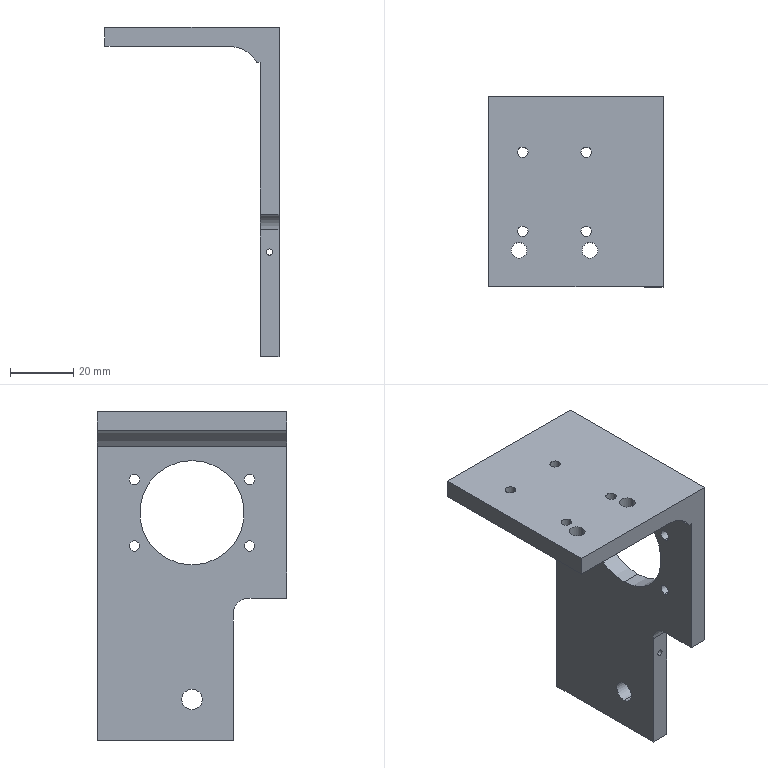Part | SolidWorks | features ICE 5, HoleWzd 3, Fillet 2, Extrusion 1 | 1 solid | 39 faces | box 55 x 60 x 104 mm | volume 45466 mm3 | cylinder 28 | plane 11 | commonest cylinder face diameters 3.3 x16 5 x4 2 x2 6.5 x2 33 x2 10 x1
STEP:
#1=CARTESIAN_POINT('',(-3.,60.,-70.));
#2=VERTEX_POINT('',#1);
#3=CARTESIAN_POINT('',(-3.,60.,-72.));
#4=VERTEX_POINT('',#3);
#5=CARTESIAN_POINT('',(-3.,60.,-71.));
#6=DIRECTION('',(0.,-1.,0.));
#7=DIRECTION('',(0.,0.,1.));
#8=AXIS2_PLACEMENT_3D('',#5,#6,#7);
#9=CIRCLE('',#8,1.);
#10=EDGE_CURVE('',#2,#4,#9,.T.);
#11=ORIENTED_EDGE('',*,*,#10,.F.);
#12=CARTESIAN_POINT('',(-3.,17.,-70.));
#13=VERTEX_POINT('',#12);
#14=CARTESIAN_POINT('',(-3.,60.001,-70.));
#15=DIRECTION('',(0.,-1.,0.));
#16=VECTOR('',#15,1000.);
#17=LINE('',#14,#16);
#18=EDGE_CURVE('',#2,#13,#17,.T.);
#19=ORIENTED_EDGE('',*,*,#18,.T.);
#20=CARTESIAN_POINT('',(-3.,17.,-72.));
#21=VERTEX_POINT('',#20);
#22=CARTESIAN_POINT('',(-3.,17.,-71.));
#23=DIRECTION('',(0.,-1.,0.));
#24=DIRECTION('',(0.,0.,-1.));
#25=AXIS2_PLACEMENT_3D('',#22,#23,#24);
#26=CIRCLE('',#25,1.);
#27=EDGE_CURVE('',#13,#21,#26,.T.);
#28=ORIENTED_EDGE('',*,*,#27,.T.);
#29=CARTESIAN_POINT('',(-3.,60.001,-72.));
#30=DIRECTION('',(0.,-1.,0.));
#31=VECTOR('',#30,1000.);
#32=LINE('',#29,#31);
#33=EDGE_CURVE('',#4,#21,#32,.T.);
#34=ORIENTED_EDGE('',*,*,#33,.F.);
#35=EDGE_LOOP('',(#11,#19,#28,#34));
#36=FACE_OUTER_BOUND('',#35,.T.);
#37=CARTESIAN_POINT('',(-3.,60.001,-71.));
#38=DIRECTION('',(0.,-1.,0.));
#39=DIRECTION('',(0.,0.,-1.));
#40=AXIS2_PLACEMENT_3D('',#37,#38,#39);
#41=CYLINDRICAL_SURFACE('',#40,1.);
#42=ADVANCED_FACE('',(#36),#41,.F.);
#43=CARTESIAN_POINT('',(-6.,30.,-87.75));
#44=VERTEX_POINT('',#43);
#45=CARTESIAN_POINT('',(-6.,30.,-94.25));
#46=VERTEX_POINT('',#45);
#47=CARTESIAN_POINT('',(-6.,30.,-91.));
#48=DIRECTION('',(1.,0.,0.));
#49=DIRECTION('',(0.,0.,-1.));
#50=AXIS2_PLACEMENT_3D('',#47,#48,#49);
#51=CIRCLE('',#50,3.25);
#52=EDGE_CURVE('',#44,#46,#51,.T.);
#53=ORIENTED_EDGE('',*,*,#52,.F.);
#54=CARTESIAN_POINT('',(0.,30.,-87.75));
#55=VERTEX_POINT('',#54);
#56=CARTESIAN_POINT('',(0.,30.,-87.75));
#57=DIRECTION('',(1.,0.,0.));
#58=VECTOR('',#57,1000.);
#59=LINE('',#56,#58);
#60=EDGE_CURVE('',#44,#55,#59,.T.);
#61=ORIENTED_EDGE('',*,*,#60,.T.);
#62=CARTESIAN_POINT('',(0.,30.,-94.25));
#63=VERTEX_POINT('',#62);
#64=CARTESIAN_POINT('',(0.,30.,-91.));
#65=DIRECTION('',(1.,0.,0.));
#66=DIRECTION('',(0.,0.,-1.));
#67=AXIS2_PLACEMENT_3D('',#64,#65,#66);
#68=CIRCLE('',#67,3.25);
#69=EDGE_CURVE('',#55,#63,#68,.T.);
#70=ORIENTED_EDGE('',*,*,#69,.T.);
#71=CARTESIAN_POINT('',(0.,30.,-94.25));
#72=DIRECTION('',(1.,0.,0.));
#73=VECTOR('',#72,1000.);
#74=LINE('',#71,#73);
#75=EDGE_CURVE('',#46,#63,#74,.T.);
#76=ORIENTED_EDGE('',*,*,#75,.F.);
#77=EDGE_LOOP('',(#53,#61,#70,#76));
#78=FACE_OUTER_BOUND('',#77,.T.);
#79=CARTESIAN_POINT('',(0.,30.,-91.));
#80=DIRECTION('',(1.,0.,0.));
#81=DIRECTION('',(0.,0.,-1.));
#82=AXIS2_PLACEMENT_3D('',#79,#80,#81);
#83=CYLINDRICAL_SURFACE('',#82,3.25);
#84=ADVANCED_FACE('',(#78),#83,.F.);
#85=CARTESIAN_POINT('',(-6.,11.813,-40.85));
#86=VERTEX_POINT('',#85);
#87=CARTESIAN_POINT('',(-6.,11.813,-44.15));
#88=VERTEX_POINT('',#87);
#89=CARTESIAN_POINT('',(-6.,11.813,-42.5));
#90=DIRECTION('',(1.,0.,0.));
#91=DIRECTION('',(0.,0.,-1.));
#92=AXIS2_PLACEMENT_3D('',#89,#90,#91);
#93=CIRCLE('',#92,1.65);
#94=EDGE_CURVE('',#86,#88,#93,.T.);
#95=ORIENTED_EDGE('',*,*,#94,.F.);
#96=CARTESIAN_POINT('',(0.,11.813,-40.85));
#97=VERTEX_POINT('',#96);
#98=CARTESIAN_POINT('',(0.,11.813,-40.85));
#99=DIRECTION('',(1.,0.,0.));
#100=VECTOR('',#99,1000.);
#101=LINE('',#98,#100);
#102=EDGE_CURVE('',#86,#97,#101,.T.);
#103=ORIENTED_EDGE('',*,*,#102,.T.);
#104=CARTESIAN_POINT('',(0.,11.813,-44.15));
#105=VERTEX_POINT('',#104);
#106=CARTESIAN_POINT('',(0.,11.813,-42.5));
#107=DIRECTION('',(1.,0.,0.));
#108=DIRECTION('',(0.,0.,-1.));
#109=AXIS2_PLACEMENT_3D('',#106,#107,#108);
#110=CIRCLE('',#109,1.65);
#111=EDGE_CURVE('',#97,#105,#110,.T.);
#112=ORIENTED_EDGE('',*,*,#111,.T.);
#113=CARTESIAN_POINT('',(0.,11.813,-44.15));
#114=DIRECTION('',(1.,0.,0.));
#115=VECTOR('',#114,1000.);
#116=LINE('',#113,#115);
#117=EDGE_CURVE('',#88,#105,#116,.T.);
#118=ORIENTED_EDGE('',*,*,#117,.F.);
#119=EDGE_LOOP('',(#95,#103,#112,#118));
#120=FACE_OUTER_BOUND('',#119,.T.);
#121=CARTESIAN_POINT('',(0.,11.813,-42.5));
#122=DIRECTION('',(1.,0.,0.));
#123=DIRECTION('',(0.,0.,-1.));
#124=AXIS2_PLACEMENT_3D('',#121,#122,#123);
#125=CYLINDRICAL_SURFACE('',#124,1.65);
#126=ADVANCED_FACE('',(#120),#125,.F.);
#127=CARTESIAN_POINT('',(-6.,48.187,-40.85));
#128=VERTEX_POINT('',#127);
#129=CARTESIAN_POINT('',(-6.,48.187,-44.15));
#130=VERTEX_POINT('',#129);
#131=CARTESIAN_POINT('',(-6.,48.187,-42.5));
#132=DIRECTION('',(1.,0.,0.));
#133=DIRECTION('',(0.,0.,-1.));
#134=AXIS2_PLACEMENT_3D('',#131,#132,#133);
#135=CIRCLE('',#134,1.65);
#136=EDGE_CURVE('',#128,#130,#135,.T.);
#137=ORIENTED_EDGE('',*,*,#136,.F.);
#138=CARTESIAN_POINT('',(0.,48.187,-40.85));
#139=VERTEX_POINT('',#138);
#140=CARTESIAN_POINT('',(0.,48.187,-40.85));
#141=DIRECTION('',(1.,0.,0.));
#142=VECTOR('',#141,1000.);
#143=LINE('',#140,#142);
#144=EDGE_CURVE('',#128,#139,#143,.T.);
#145=ORIENTED_EDGE('',*,*,#144,.T.);
#146=CARTESIAN_POINT('',(0.,48.187,-44.15));
#147=VERTEX_POINT('',#146);
#148=CARTESIAN_POINT('',(0.,48.187,-42.5));
#149=DIRECTION('',(1.,0.,0.));
#150=DIRECTION('',(0.,0.,-1.));
#151=AXIS2_PLACEMENT_3D('',#148,#149,#150);
#152=CIRCLE('',#151,1.65);
#153=EDGE_CURVE('',#139,#147,#152,.T.);
#154=ORIENTED_EDGE('',*,*,#153,.T.);
#155=CARTESIAN_POINT('',(0.,48.187,-44.15));
#156=DIRECTION('',(1.,0.,0.));
#157=VECTOR('',#156,1000.);
#158=LINE('',#155,#157);
#159=EDGE_CURVE('',#130,#147,#158,.T.);
#160=ORIENTED_EDGE('',*,*,#159,.F.);
#161=EDGE_LOOP('',(#137,#145,#154,#160));
#162=FACE_OUTER_BOUND('',#161,.T.);
#163=CARTESIAN_POINT('',(0.,48.187,-42.5));
#164=DIRECTION('',(1.,0.,0.));
#165=DIRECTION('',(0.,0.,-1.));
#166=AXIS2_PLACEMENT_3D('',#163,#164,#165);
#167=CYLINDRICAL_SURFACE('',#166,1.65);
#168=ADVANCED_FACE('',(#162),#167,.F.);
#169=CARTESIAN_POINT('',(-6.,48.187,-19.85));
#170=VERTEX_POINT('',#169);
#171=CARTESIAN_POINT('',(-6.,48.187,-23.15));
#172=VERTEX_POINT('',#171);
#173=CARTESIAN_POINT('',(-6.,48.187,-21.5));
#174=DIRECTION('',(1.,0.,0.));
#175=DIRECTION('',(0.,0.,-1.));
#176=AXIS2_PLACEMENT_3D('',#173,#174,#175);
#177=CIRCLE('',#176,1.65);
#178=EDGE_CURVE('',#170,#172,#177,.T.);
#179=ORIENTED_EDGE('',*,*,#178,.F.);
#180=CARTESIAN_POINT('',(0.,48.187,-19.85));
#181=VERTEX_POINT('',#180);
#182=CARTESIAN_POINT('',(0.,48.187,-19.85));
#183=DIRECTION('',(1.,0.,0.));
#184=VECTOR('',#183,1000.);
#185=LINE('',#182,#184);
#186=EDGE_CURVE('',#170,#181,#185,.T.);
#187=ORIENTED_EDGE('',*,*,#186,.T.);
#188=CARTESIAN_POINT('',(0.,48.187,-23.15));
#189=VERTEX_POINT('',#188);
#190=CARTESIAN_POINT('',(0.,48.187,-21.5));
#191=DIRECTION('',(1.,0.,0.));
#192=DIRECTION('',(0.,0.,-1.));
#193=AXIS2_PLACEMENT_3D('',#190,#191,#192);
#194=CIRCLE('',#193,1.65);
#195=EDGE_CURVE('',#181,#189,#194,.T.);
#196=ORIENTED_EDGE('',*,*,#195,.T.);
#197=CARTESIAN_POINT('',(0.,48.187,-23.15));
#198=DIRECTION('',(1.,0.,0.));
#199=VECTOR('',#198,1000.);
#200=LINE('',#197,#199);
#201=EDGE_CURVE('',#172,#189,#200,.T.);
#202=ORIENTED_EDGE('',*,*,#201,.F.);
#203=EDGE_LOOP('',(#179,#187,#196,#202));
#204=FACE_OUTER_BOUND('',#203,.T.);
#205=CARTESIAN_POINT('',(0.,48.187,-21.5));
#206=DIRECTION('',(1.,0.,0.));
#207=DIRECTION('',(0.,0.,-1.));
#208=AXIS2_PLACEMENT_3D('',#205,#206,#207);
#209=CYLINDRICAL_SURFACE('',#208,1.65);
#210=ADVANCED_FACE('',(#204),#209,.F.);
#211=CARTESIAN_POINT('',(-6.,11.813,-19.85));
#212=VERTEX_POINT('',#211);
#213=CARTESIAN_POINT('',(-6.,11.813,-23.15));
#214=VERTEX_POINT('',#213);
#215=CARTESIAN_POINT('',(-6.,11.813,-21.5));
#216=DIRECTION('',(1.,0.,0.));
#217=DIRECTION('',(0.,0.,-1.));
#218=AXIS2_PLACEMENT_3D('',#215,#216,#217);
#219=CIRCLE('',#218,1.65);
#220=EDGE_CURVE('',#212,#214,#219,.T.);
#221=ORIENTED_EDGE('',*,*,#220,.F.);
#222=CARTESIAN_POINT('',(0.,11.813,-19.85));
#223=VERTEX_POINT('',#222);
#224=CARTESIAN_POINT('',(0.,11.813,-19.85));
#225=DIRECTION('',(1.,0.,0.));
#226=VECTOR('',#225,1000.);
#227=LINE('',#224,#226);
#228=EDGE_CURVE('',#212,#223,#227,.T.);
#229=ORIENTED_EDGE('',*,*,#228,.T.);
#230=CARTESIAN_POINT('',(0.,11.813,-23.15));
#231=VERTEX_POINT('',#230);
#232=CARTESIAN_POINT('',(0.,11.813,-21.5));
#233=DIRECTION('',(1.,0.,0.));
#234=DIRECTION('',(0.,0.,-1.));
#235=AXIS2_PLACEMENT_3D('',#232,#233,#234);
#236=CIRCLE('',#235,1.65);
#237=EDGE_CURVE('',#223,#231,#236,.T.);
#238=ORIENTED_EDGE('',*,*,#237,.T.);
#239=CARTESIAN_POINT('',(0.,11.813,-23.15));
#240=DIRECTION('',(1.,0.,0.));
#241=VECTOR('',#240,1000.);
#242=LINE('',#239,#241);
#243=EDGE_CURVE('',#214,#231,#242,.T.);
#244=ORIENTED_EDGE('',*,*,#243,.F.);
#245=EDGE_LOOP('',(#221,#229,#238,#244));
#246=FACE_OUTER_BOUND('',#245,.T.);
#247=CARTESIAN_POINT('',(0.,11.813,-21.5));
#248=DIRECTION('',(1.,0.,0.));
#249=DIRECTION('',(0.,0.,-1.));
#250=AXIS2_PLACEMENT_3D('',#247,#248,#249);
#251=CYLINDRICAL_SURFACE('',#250,1.65);
#252=ADVANCED_FACE('',(#246),#251,.F.);
#253=CARTESIAN_POINT('',(-6.,30.,-15.5));
#254=VERTEX_POINT('',#253);
#255=CARTESIAN_POINT('',(-6.,30.,-48.5));
#256=VERTEX_POINT('',#255);
#257=CARTESIAN_POINT('',(-6.,30.,-32.));
#258=DIRECTION('',(1.,0.,0.));
#259=DIRECTION('',(0.,0.,-1.));
#260=AXIS2_PLACEMENT_3D('',#257,#258,#259);
#261=CIRCLE('',#260,16.5);
#262=EDGE_CURVE('',#254,#256,#261,.T.);
#263=ORIENTED_EDGE('',*,*,#262,.F.);
#264=CARTESIAN_POINT('',(0.,30.,-15.5));
#265=VERTEX_POINT('',#264);
#266=CARTESIAN_POINT('',(-55.,30.,-15.5));
#267=DIRECTION('',(1.,0.,0.));
#268=VECTOR('',#267,1000.);
#269=LINE('',#266,#268);
#270=EDGE_CURVE('',#254,#265,#269,.T.);
#271=ORIENTED_EDGE('',*,*,#270,.T.);
#272=CARTESIAN_POINT('',(0.,30.,-48.5));
#273=VERTEX_POINT('',#272);
#274=CARTESIAN_POINT('',(0.,30.,-32.));
#275=DIRECTION('',(1.,0.,0.));
#276=DIRECTION('',(0.,0.,-1.));
#277=AXIS2_PLACEMENT_3D('',#274,#275,#276);
#278=CIRCLE('',#277,16.5);
#279=EDGE_CURVE('',#265,#273,#278,.T.);
#280=ORIENTED_EDGE('',*,*,#279,.T.);
#281=CARTESIAN_POINT('',(-55.,30.,-48.5));
#282=DIRECTION('',(1.,0.,0.));
#283=VECTOR('',#282,1000.);
#284=LINE('',#281,#283);
#285=EDGE_CURVE('',#256,#273,#284,.T.);
#286=ORIENTED_EDGE('',*,*,#285,.F.);
#287=EDGE_LOOP('',(#263,#271,#280,#286));
#288=FACE_OUTER_BOUND('',#287,.T.);
#289=CARTESIAN_POINT('',(-55.,30.,-32.));
#290=DIRECTION('',(1.,0.,0.));
#291=DIRECTION('',(0.,0.,-1.));
#292=AXIS2_PLACEMENT_3D('',#289,#290,#291);
#293=CYLINDRICAL_SURFACE('',#292,16.5);
#294=ADVANCED_FACE('',(#288),#293,.F.);
#295=CARTESIAN_POINT('',(-25.6,11.5,-6.));
#296=VERTEX_POINT('',#295);
#297=CARTESIAN_POINT('',(-20.6,11.5,-6.));
#298=VERTEX_POINT('',#297);
#299=CARTESIAN_POINT('',(-23.1,11.5,-6.));
#300=DIRECTION('',(0.,0.,1.));
#301=DIRECTION('',(1.,0.,0.));
#302=AXIS2_PLACEMENT_3D('',#299,#300,#301);
#303=CIRCLE('',#302,2.5);
#304=EDGE_CURVE('',#296,#298,#303,.T.);
#305=ORIENTED_EDGE('',*,*,#304,.F.);
#306=CARTESIAN_POINT('',(-25.6,11.5,0.));
#307=VERTEX_POINT('',#306);
#308=CARTESIAN_POINT('',(-25.6,11.5,-104.));
#309=DIRECTION('',(0.,0.,1.));
#310=VECTOR('',#309,1000.);
#311=LINE('',#308,#310);
#312=EDGE_CURVE('',#296,#307,#311,.T.);
#313=ORIENTED_EDGE('',*,*,#312,.T.);
#314=CARTESIAN_POINT('',(-20.6,11.5,0.));
#315=VERTEX_POINT('',#314);
#316=CARTESIAN_POINT('',(-23.1,11.5,0.));
#317=DIRECTION('',(0.,0.,1.));
#318=DIRECTION('',(1.,0.,0.));
#319=AXIS2_PLACEMENT_3D('',#316,#317,#318);
#320=CIRCLE('',#319,2.5);
#321=EDGE_CURVE('',#307,#315,#320,.T.);
#322=ORIENTED_EDGE('',*,*,#321,.T.);
#323=CARTESIAN_POINT('',(-20.6,11.5,-104.));
#324=DIRECTION('',(0.,0.,1.));
#325=VECTOR('',#324,1000.);
#326=LINE('',#323,#325);
#327=EDGE_CURVE('',#298,#315,#326,.T.);
#328=ORIENTED_EDGE('',*,*,#327,.F.);
#329=EDGE_LOOP('',(#305,#313,#322,#328));
#330=FACE_OUTER_BOUND('',#329,.T.);
#331=CARTESIAN_POINT('',(-23.1,11.5,-104.));
#332=DIRECTION('',(0.,0.,1.));
#333=DIRECTION('',(1.,0.,0.));
#334=AXIS2_PLACEMENT_3D('',#331,#332,#333);
#335=CYLINDRICAL_SURFACE('',#334,2.5);
#336=ADVANCED_FACE('',(#330),#335,.F.);
#337=CARTESIAN_POINT('',(-48.,11.5,-6.));
#338=VERTEX_POINT('',#337);
#339=CARTESIAN_POINT('',(-43.,11.5,-6.));
#340=VERTEX_POINT('',#339);
#341=CARTESIAN_POINT('',(-45.5,11.5,-6.));
#342=DIRECTION('',(0.,0.,1.));
#343=DIRECTION('',(1.,0.,0.));
#344=AXIS2_PLACEMENT_3D('',#341,#342,#343);
#345=CIRCLE('',#344,2.5);
#346=EDGE_CURVE('',#338,#340,#345,.T.);
#347=ORIENTED_EDGE('',*,*,#346,.F.);
#348=CARTESIAN_POINT('',(-48.,11.5,0.));
#349=VERTEX_POINT('',#348);
#350=CARTESIAN_POINT('',(-48.,11.5,-104.));
#351=DIRECTION('',(0.,0.,1.));
#352=VECTOR('',#351,1000.);
#353=LINE('',#350,#352);
#354=EDGE_CURVE('',#338,#349,#353,.T.);
#355=ORIENTED_EDGE('',*,*,#354,.T.);
#356=CARTESIAN_POINT('',(-43.,11.5,0.));
#357=VERTEX_POINT('',#356);
#358=CARTESIAN_POINT('',(-45.5,11.5,0.));
#359=DIRECTION('',(0.,0.,1.));
#360=DIRECTION('',(1.,0.,0.));
#361=AXIS2_PLACEMENT_3D('',#358,#359,#360);
#362=CIRCLE('',#361,2.5);
#363=EDGE_CURVE('',#349,#357,#362,.T.);
#364=ORIENTED_EDGE('',*,*,#363,.T.);
#365=CARTESIAN_POINT('',(-43.,11.5,-104.));
#366=DIRECTION('',(0.,0.,1.));
#367=VECTOR('',#366,1000.);
#368=LINE('',#365,#367);
#369=EDGE_CURVE('',#340,#357,#368,.T.);
#370=ORIENTED_EDGE('',*,*,#369,.F.);
#371=EDGE_LOOP('',(#347,#355,#364,#370));
#372=FACE_OUTER_BOUND('',#371,.T.);
#373=CARTESIAN_POINT('',(-45.5,11.5,-104.));
#374=DIRECTION('',(0.,0.,1.));
#375=DIRECTION('',(1.,0.,0.));
#376=AXIS2_PLACEMENT_3D('',#373,#374,#375);
#377=CYLINDRICAL_SURFACE('',#376,2.5);
#378=ADVANCED_FACE('',(#372),#377,.F.);
#379=CARTESIAN_POINT('',(-45.95,42.5,-6.));
#380=VERTEX_POINT('',#379);
#381=CARTESIAN_POINT('',(-42.65,42.5,-6.));
#382=VERTEX_POINT('',#381);
#383=CARTESIAN_POINT('',(-44.3,42.5,-6.));
#384=DIRECTION('',(0.,0.,1.));
#385=DIRECTION('',(1.,0.,0.));
#386=AXIS2_PLACEMENT_3D('',#383,#384,#385);
#387=CIRCLE('',#386,1.65);
#388=EDGE_CURVE('',#380,#382,#387,.T.);
#389=ORIENTED_EDGE('',*,*,#388,.F.);
#390=CARTESIAN_POINT('',(-45.95,42.5,0.));
#391=VERTEX_POINT('',#390);
#392=CARTESIAN_POINT('',(-45.95,42.5,0.));
#393=DIRECTION('',(0.,0.,1.));
#394=VECTOR('',#393,1000.);
#395=LINE('',#392,#394);
#396=EDGE_CURVE('',#380,#391,#395,.T.);
#397=ORIENTED_EDGE('',*,*,#396,.T.);
#398=CARTESIAN_POINT('',(-42.65,42.5,0.));
#399=VERTEX_POINT('',#398);
#400=CARTESIAN_POINT('',(-44.3,42.5,0.));
#401=DIRECTION('',(0.,0.,1.));
#402=DIRECTION('',(1.,0.,0.));
#403=AXIS2_PLACEMENT_3D('',#400,#401,#402);
#404=CIRCLE('',#403,1.65);
#405=EDGE_CURVE('',#391,#399,#404,.T.);
#406=ORIENTED_EDGE('',*,*,#405,.T.);
#407=CARTESIAN_POINT('',(-42.65,42.5,0.));
#408=DIRECTION('',(0.,0.,1.));
#409=VECTOR('',#408,1000.);
#410=LINE('',#407,#409);
#411=EDGE_CURVE('',#382,#399,#410,.T.);
#412=ORIENTED_EDGE('',*,*,#411,.F.);
#413=EDGE_LOOP('',(#389,#397,#406,#412));
#414=FACE_OUTER_BOUND('',#413,.T.);
#415=CARTESIAN_POINT('',(-44.3,42.5,0.));
#416=DIRECTION('',(0.,0.,1.));
#417=DIRECTION('',(1.,0.,0.));
#418=AXIS2_PLACEMENT_3D('',#415,#416,#417);
#419=CYLINDRICAL_SURFACE('',#418,1.65);
#420=ADVANCED_FACE('',(#414),#419,.F.);
#421=CARTESIAN_POINT('',(-25.95,42.5,-6.));
#422=VERTEX_POINT('',#421);
#423=CARTESIAN_POINT('',(-22.65,42.5,-6.));
#424=VERTEX_POINT('',#423);
#425=CARTESIAN_POINT('',(-24.3,42.5,-6.));
#426=DIRECTION('',(0.,0.,1.));
#427=DIRECTION('',(1.,0.,0.));
#428=AXIS2_PLACEMENT_3D('',#425,#426,#427);
#429=CIRCLE('',#428,1.65);
#430=EDGE_CURVE('',#422,#424,#429,.T.);
#431=ORIENTED_EDGE('',*,*,#430,.F.);
#432=CARTESIAN_POINT('',(-25.95,42.5,0.));
#433=VERTEX_POINT('',#432);
#434=CARTESIAN_POINT('',(-25.95,42.5,0.));
#435=DIRECTION('',(0.,0.,1.));
#436=VECTOR('',#435,1000.);
#437=LINE('',#434,#436);
#438=EDGE_CURVE('',#422,#433,#437,.T.);
#439=ORIENTED_EDGE('',*,*,#438,.T.);
#440=CARTESIAN_POINT('',(-22.65,42.5,0.));
#441=VERTEX_POINT('',#440);
#442=CARTESIAN_POINT('',(-24.3,42.5,0.));
#443=DIRECTION('',(0.,0.,1.));
#444=DIRECTION('',(1.,0.,0.));
#445=AXIS2_PLACEMENT_3D('',#442,#443,#444);
#446=CIRCLE('',#445,1.65);
#447=EDGE_CURVE('',#433,#441,#446,.T.);
#448=ORIENTED_EDGE('',*,*,#447,.T.);
#449=CARTESIAN_POINT('',(-22.65,42.5,0.));
#450=DIRECTION('',(0.,0.,1.));
#451=VECTOR('',#450,1000.);
#452=LINE('',#449,#451);
#453=EDGE_CURVE('',#424,#441,#452,.T.);
#454=ORIENTED_EDGE('',*,*,#453,.F.);
#455=EDGE_LOOP('',(#431,#439,#448,#454));
#456=FACE_OUTER_BOUND('',#455,.T.);
#457=CARTESIAN_POINT('',(-24.3,42.5,0.));
#458=DIRECTION('',(0.,0.,1.));
#459=DIRECTION('',(1.,0.,0.));
#460=AXIS2_PLACEMENT_3D('',#457,#458,#459);
#461=CYLINDRICAL_SURFACE('',#460,1.65);
#462=ADVANCED_FACE('',(#456),#461,.F.);
#463=CARTESIAN_POINT('',(-25.95,17.5,-6.));
#464=VERTEX_POINT('',#463);
#465=CARTESIAN_POINT('',(-22.65,17.5,-6.));
#466=VERTEX_POINT('',#465);
#467=CARTESIAN_POINT('',(-24.3,17.5,-6.));
#468=DIRECTION('',(0.,0.,1.));
#469=DIRECTION('',(1.,0.,0.));
#470=AXIS2_PLACEMENT_3D('',#467,#468,#469);
#471=CIRCLE('',#470,1.65);
#472=EDGE_CURVE('',#464,#466,#471,.T.);
#473=ORIENTED_EDGE('',*,*,#472,.F.);
#474=CARTESIAN_POINT('',(-25.95,17.5,0.));
#475=VERTEX_POINT('',#474);
#476=CARTESIAN_POINT('',(-25.95,17.5,0.));
#477=DIRECTION('',(0.,0.,1.));
#478=VECTOR('',#477,1000.);
#479=LINE('',#476,#478);
#480=EDGE_CURVE('',#464,#475,#479,.T.);
#481=ORIENTED_EDGE('',*,*,#480,.T.);
#482=CARTESIAN_POINT('',(-22.65,17.5,0.));
#483=VERTEX_POINT('',#482);
#484=CARTESIAN_POINT('',(-24.3,17.5,0.));
#485=DIRECTION('',(0.,0.,1.));
#486=DIRECTION('',(1.,0.,0.));
#487=AXIS2_PLACEMENT_3D('',#484,#485,#486);
#488=CIRCLE('',#487,1.65);
#489=EDGE_CURVE('',#475,#483,#488,.T.);
#490=ORIENTED_EDGE('',*,*,#489,.T.);
#491=CARTESIAN_POINT('',(-22.65,17.5,0.));
#492=DIRECTION('',(0.,0.,1.));
#493=VECTOR('',#492,1000.);
#494=LINE('',#491,#493);
#495=EDGE_CURVE('',#466,#483,#494,.T.);
#496=ORIENTED_EDGE('',*,*,#495,.F.);
#497=EDGE_LOOP('',(#473,#481,#490,#496));
#498=FACE_OUTER_BOUND('',#497,.T.);
#499=CARTESIAN_POINT('',(-24.3,17.5,0.));
#500=DIRECTION('',(0.,0.,1.));
#501=DIRECTION('',(1.,0.,0.));
#502=AXIS2_PLACEMENT_3D('',#499,#500,#501);
#503=CYLINDRICAL_SURFACE('',#502,1.65);
#504=ADVANCED_FACE('',(#498),#503,.F.);
#505=CARTESIAN_POINT('',(-45.95,17.5,-6.));
#506=VERTEX_POINT('',#505);
#507=CARTESIAN_POINT('',(-42.65,17.5,-6.));
#508=VERTEX_POINT('',#507);
#509=CARTESIAN_POINT('',(-44.3,17.5,-6.));
#510=DIRECTION('',(0.,0.,1.));
#511=DIRECTION('',(1.,0.,0.));
#512=AXIS2_PLACEMENT_3D('',#509,#510,#511);
#513=CIRCLE('',#512,1.65);
#514=EDGE_CURVE('',#506,#508,#513,.T.);
#515=ORIENTED_EDGE('',*,*,#514,.F.);
#516=CARTESIAN_POINT('',(-45.95,17.5,0.));
#517=VERTEX_POINT('',#516);
#518=CARTESIAN_POINT('',(-45.95,17.5,0.));
#519=DIRECTION('',(0.,0.,1.));
#520=VECTOR('',#519,1000.);
#521=LINE('',#518,#520);
#522=EDGE_CURVE('',#506,#517,#521,.T.);
#523=ORIENTED_EDGE('',*,*,#522,.T.);
#524=CARTESIAN_POINT('',(-42.65,17.5,0.));
#525=VERTEX_POINT('',#524);
#526=CARTESIAN_POINT('',(-44.3,17.5,0.));
#527=DIRECTION('',(0.,0.,1.));
#528=DIRECTION('',(1.,0.,0.));
#529=AXIS2_PLACEMENT_3D('',#526,#527,#528);
#530=CIRCLE('',#529,1.65);
#531=EDGE_CURVE('',#517,#525,#530,.T.);
#532=ORIENTED_EDGE('',*,*,#531,.T.);
#533=CARTESIAN_POINT('',(-42.65,17.5,0.));
#534=DIRECTION('',(0.,0.,1.));
#535=VECTOR('',#534,1000.);
#536=LINE('',#533,#535);
#537=EDGE_CURVE('',#508,#525,#536,.T.);
#538=ORIENTED_EDGE('',*,*,#537,.F.);
#539=EDGE_LOOP('',(#515,#523,#532,#538));
#540=FACE_OUTER_BOUND('',#539,.T.);
#541=CARTESIAN_POINT('',(-44.3,17.5,0.));
#542=DIRECTION('',(0.,0.,1.));
#543=DIRECTION('',(1.,0.,0.));
#544=AXIS2_PLACEMENT_3D('',#541,#542,#543);
#545=CYLINDRICAL_SURFACE('',#544,1.65);
#546=ADVANCED_FACE('',(#540),#545,.F.);
#547=CARTESIAN_POINT('',(-55.,0.,-6.));
#548=VERTEX_POINT('',#547);
#549=CARTESIAN_POINT('',(-55.,0.,0.));
#550=VERTEX_POINT('',#549);
#551=CARTESIAN_POINT('',(-55.,0.,-6.));
#552=DIRECTION('',(0.,0.,1.));
#553=VECTOR('',#552,1000.);
#554=LINE('',#551,#553);
#555=EDGE_CURVE('',#548,#550,#554,.T.);
#556=ORIENTED_EDGE('',*,*,#555,.T.);
#557=CARTESIAN_POINT('',(-55.,60.,0.));
#558=VERTEX_POINT('',#557);
#559=CARTESIAN_POINT('',(-55.,60.,0.));
#560=DIRECTION('',(0.,-1.,0.));
#561=VECTOR('',#560,1000.);
#562=LINE('',#559,#561);
#563=EDGE_CURVE('',#558,#550,#562,.T.);
#564=ORIENTED_EDGE('',*,*,#563,.F.);
#565=CARTESIAN_POINT('',(-55.,60.,-6.));
#566=VERTEX_POINT('',#565);
#567=CARTESIAN_POINT('',(-55.,60.,-6.));
#568=DIRECTION('',(0.,0.,1.));
#569=VECTOR('',#568,1000.);
#570=LINE('',#567,#569);
#571=EDGE_CURVE('',#566,#558,#570,.T.);
#572=ORIENTED_EDGE('',*,*,#571,.F.);
#573=CARTESIAN_POINT('',(-55.,60.,-6.));
#574=DIRECTION('',(0.,-1.,0.));
#575=VECTOR('',#574,1000.);
#576=LINE('',#573,#575);
#577=EDGE_CURVE('',#566,#548,#576,.T.);
#578=ORIENTED_EDGE('',*,*,#577,.T.);
#579=EDGE_LOOP('',(#556,#564,#572,#578));
#580=FACE_OUTER_BOUND('',#579,.T.);
#581=CARTESIAN_POINT('',(-55.,60.,-6.));
#582=DIRECTION('',(1.,0.,0.));
#583=DIRECTION('',(0.,0.,-1.));
#584=AXIS2_PLACEMENT_3D('',#581,#582,#583);
#585=PLANE('',#584);
#586=ADVANCED_FACE('',(#580),#585,.F.);
#587=CARTESIAN_POINT('',(-23.1,11.5,0.));
#588=DIRECTION('',(0.,0.,1.));
#589=DIRECTION('',(1.,0.,0.));
#590=AXIS2_PLACEMENT_3D('',#587,#588,#589);
#591=CIRCLE('',#590,2.5);
#592=EDGE_CURVE('',#315,#307,#591,.T.);
#593=ORIENTED_EDGE('',*,*,#592,.F.);
#594=ORIENTED_EDGE('',*,*,#321,.F.);
#595=EDGE_LOOP('',(#593,#594));
#596=FACE_BOUND('',#595,.T.);
#597=CARTESIAN_POINT('',(-45.5,11.5,0.));
#598=DIRECTION('',(0.,0.,1.));
#599=DIRECTION('',(1.,0.,0.));
#600=AXIS2_PLACEMENT_3D('',#597,#598,#599);
#601=CIRCLE('',#600,2.5);
#602=EDGE_CURVE('',#357,#349,#601,.T.);
#603=ORIENTED_EDGE('',*,*,#602,.F.);
#604=ORIENTED_EDGE('',*,*,#363,.F.);
#605=EDGE_LOOP('',(#603,#604));
#606=FACE_BOUND('',#605,.T.);
#607=CARTESIAN_POINT('',(-44.3,42.5,0.));
#608=DIRECTION('',(0.,0.,1.));
#609=DIRECTION('',(1.,0.,0.));
#610=AXIS2_PLACEMENT_3D('',#607,#608,#609);
#611=CIRCLE('',#610,1.65);
#612=EDGE_CURVE('',#399,#391,#611,.T.);
#613=ORIENTED_EDGE('',*,*,#612,.F.);
#614=ORIENTED_EDGE('',*,*,#405,.F.);
#615=EDGE_LOOP('',(#613,#614));
#616=FACE_BOUND('',#615,.T.);
#617=CARTESIAN_POINT('',(-24.3,42.5,0.));
#618=DIRECTION('',(0.,0.,1.));
#619=DIRECTION('',(1.,0.,0.));
#620=AXIS2_PLACEMENT_3D('',#617,#618,#619);
#621=CIRCLE('',#620,1.65);
#622=EDGE_CURVE('',#441,#433,#621,.T.);
#623=ORIENTED_EDGE('',*,*,#622,.F.);
#624=ORIENTED_EDGE('',*,*,#447,.F.);
#625=EDGE_LOOP('',(#623,#624));
#626=FACE_BOUND('',#625,.T.);
#627=CARTESIAN_POINT('',(-24.3,17.5,0.));
#628=DIRECTION('',(0.,0.,1.));
#629=DIRECTION('',(1.,0.,0.));
#630=AXIS2_PLACEMENT_3D('',#627,#628,#629);
#631=CIRCLE('',#630,1.65);
#632=EDGE_CURVE('',#483,#475,#631,.T.);
#633=ORIENTED_EDGE('',*,*,#632,.F.);
#634=ORIENTED_EDGE('',*,*,#489,.F.);
#635=EDGE_LOOP('',(#633,#634));
#636=FACE_BOUND('',#635,.T.);
#637=CARTESIAN_POINT('',(-44.3,17.5,0.));
#638=DIRECTION('',(0.,0.,1.));
#639=DIRECTION('',(1.,0.,0.));
#640=AXIS2_PLACEMENT_3D('',#637,#638,#639);
#641=CIRCLE('',#640,1.65);
#642=EDGE_CURVE('',#525,#517,#641,.T.);
#643=ORIENTED_EDGE('',*,*,#642,.F.);
#644=ORIENTED_EDGE('',*,*,#531,.F.);
#645=EDGE_LOOP('',(#643,#644));
#646=FACE_BOUND('',#645,.T.);
#647=CARTESIAN_POINT('',(0.,0.,0.));
#648=VERTEX_POINT('',#647);
#649=CARTESIAN_POINT('',(-55.,0.,0.));
#650=DIRECTION('',(1.,0.,0.));
#651=VECTOR('',#650,1000.);
#652=LINE('',#649,#651);
#653=EDGE_CURVE('',#550,#648,#652,.T.);
#654=ORIENTED_EDGE('',*,*,#653,.T.);
#655=CARTESIAN_POINT('',(0.,60.,0.));
#656=VERTEX_POINT('',#655);
#657=CARTESIAN_POINT('',(0.,60.,0.));
#658=DIRECTION('',(0.,-1.,0.));
#659=VECTOR('',#658,1000.);
#660=LINE('',#657,#659);
#661=EDGE_CURVE('',#656,#648,#660,.T.);
#662=ORIENTED_EDGE('',*,*,#661,.F.);
#663=CARTESIAN_POINT('',(-55.,60.,0.));
#664=DIRECTION('',(1.,0.,0.));
#665=VECTOR('',#664,1000.);
#666=LINE('',#663,#665);
#667=EDGE_CURVE('',#558,#656,#666,.T.);
#668=ORIENTED_EDGE('',*,*,#667,.F.);
#669=ORIENTED_EDGE('',*,*,#563,.T.);
#670=EDGE_LOOP('',(#654,#662,#668,#669));
#671=FACE_OUTER_BOUND('',#670,.T.);
#672=CARTESIAN_POINT('',(-55.,60.,0.));
#673=DIRECTION('',(0.,0.,-1.));
#674=DIRECTION('',(-1.,0.,0.));
#675=AXIS2_PLACEMENT_3D('',#672,#673,#674);
#676=PLANE('',#675);
#677=ADVANCED_FACE('',(#596,#606,#616,#626,#636,#646,#671),#676,.F.);
#678=CARTESIAN_POINT('',(0.,30.,-91.));
#679=DIRECTION('',(1.,0.,0.));
#680=DIRECTION('',(0.,0.,-1.));
#681=AXIS2_PLACEMENT_3D('',#678,#679,#680);
#682=CIRCLE('',#681,3.25);
#683=EDGE_CURVE('',#63,#55,#682,.T.);
#684=ORIENTED_EDGE('',*,*,#683,.F.);
#685=ORIENTED_EDGE('',*,*,#69,.F.);
#686=EDGE_LOOP('',(#684,#685));
#687=FACE_BOUND('',#686,.T.);
#688=CARTESIAN_POINT('',(0.,11.813,-42.5));
#689=DIRECTION('',(1.,0.,0.));
#690=DIRECTION('',(0.,0.,-1.));
#691=AXIS2_PLACEMENT_3D('',#688,#689,#690);
#692=CIRCLE('',#691,1.65);
#693=EDGE_CURVE('',#105,#97,#692,.T.);
#694=ORIENTED_EDGE('',*,*,#693,.F.);
#695=ORIENTED_EDGE('',*,*,#111,.F.);
#696=EDGE_LOOP('',(#694,#695));
#697=FACE_BOUND('',#696,.T.);
#698=CARTESIAN_POINT('',(0.,48.187,-42.5));
#699=DIRECTION('',(1.,0.,0.));
#700=DIRECTION('',(0.,0.,-1.));
#701=AXIS2_PLACEMENT_3D('',#698,#699,#700);
#702=CIRCLE('',#701,1.65);
#703=EDGE_CURVE('',#147,#139,#702,.T.);
#704=ORIENTED_EDGE('',*,*,#703,.F.);
#705=ORIENTED_EDGE('',*,*,#153,.F.);
#706=EDGE_LOOP('',(#704,#705));
#707=FACE_BOUND('',#706,.T.);
#708=CARTESIAN_POINT('',(0.,48.187,-21.5));
#709=DIRECTION('',(1.,0.,0.));
#710=DIRECTION('',(0.,0.,-1.));
#711=AXIS2_PLACEMENT_3D('',#708,#709,#710);
#712=CIRCLE('',#711,1.65);
#713=EDGE_CURVE('',#189,#181,#712,.T.);
#714=ORIENTED_EDGE('',*,*,#713,.F.);
#715=ORIENTED_EDGE('',*,*,#195,.F.);
#716=EDGE_LOOP('',(#714,#715));
#717=FACE_BOUND('',#716,.T.);
#718=CARTESIAN_POINT('',(0.,11.813,-21.5));
#719=DIRECTION('',(1.,0.,0.));
#720=DIRECTION('',(0.,0.,-1.));
#721=AXIS2_PLACEMENT_3D('',#718,#719,#720);
#722=CIRCLE('',#721,1.65);
#723=EDGE_CURVE('',#231,#223,#722,.T.);
#724=ORIENTED_EDGE('',*,*,#723,.F.);
#725=ORIENTED_EDGE('',*,*,#237,.F.);
#726=EDGE_LOOP('',(#724,#725));
#727=FACE_BOUND('',#726,.T.);
#728=CARTESIAN_POINT('',(0.,30.,-32.));
#729=DIRECTION('',(1.,0.,0.));
#730=DIRECTION('',(0.,0.,-1.));
#731=AXIS2_PLACEMENT_3D('',#728,#729,#730);
#732=CIRCLE('',#731,16.5);
#733=EDGE_CURVE('',#273,#265,#732,.T.);
#734=ORIENTED_EDGE('',*,*,#733,.F.);
#735=ORIENTED_EDGE('',*,*,#279,.F.);
#736=EDGE_LOOP('',(#734,#735));
#737=FACE_BOUND('',#736,.T.);
#738=CARTESIAN_POINT('',(0.,0.,-59.));
#739=VERTEX_POINT('',#738);
#740=CARTESIAN_POINT('',(0.,0.,0.));
#741=DIRECTION('',(0.,0.,-1.));
#742=VECTOR('',#741,1000.);
#743=LINE('',#740,#742);
#744=EDGE_CURVE('',#648,#739,#743,.T.);
#745=ORIENTED_EDGE('',*,*,#744,.T.);
#746=CARTESIAN_POINT('',(0.,12.,-59.));
#747=VERTEX_POINT('',#746);
#748=CARTESIAN_POINT('',(0.,0.,-59.));
#749=DIRECTION('',(0.,-1.,0.));
#750=VECTOR('',#749,1000.);
#751=LINE('',#748,#750);
#752=EDGE_CURVE('',#747,#739,#751,.T.);
#753=ORIENTED_EDGE('',*,*,#752,.F.);
#754=CARTESIAN_POINT('',(0.,17.,-64.));
#755=VERTEX_POINT('',#754);
#756=CARTESIAN_POINT('',(0.,12.,-64.));
#757=DIRECTION('',(-1.,0.,0.));
#758=DIRECTION('',(0.,0.,1.));
#759=AXIS2_PLACEMENT_3D('',#756,#757,#758);
#760=CIRCLE('',#759,5.);
#761=EDGE_CURVE('',#747,#755,#760,.T.);
#762=ORIENTED_EDGE('',*,*,#761,.T.);
#763=CARTESIAN_POINT('',(0.,17.,-104.));
#764=VERTEX_POINT('',#763);
#765=CARTESIAN_POINT('',(0.,17.,-104.));
#766=DIRECTION('',(0.,0.,1.));
#767=VECTOR('',#766,1000.);
#768=LINE('',#765,#767);
#769=EDGE_CURVE('',#764,#755,#768,.T.);
#770=ORIENTED_EDGE('',*,*,#769,.F.);
#771=CARTESIAN_POINT('',(0.,60.,-104.));
#772=VERTEX_POINT('',#771);
#773=CARTESIAN_POINT('',(0.,60.,-104.));
#774=DIRECTION('',(0.,-1.,0.));
#775=VECTOR('',#774,1000.);
#776=LINE('',#773,#775);
#777=EDGE_CURVE('',#772,#764,#776,.T.);
#778=ORIENTED_EDGE('',*,*,#777,.F.);
#779=CARTESIAN_POINT('',(0.,60.,0.));
#780=DIRECTION('',(0.,0.,-1.));
#781=VECTOR('',#780,1000.);
#782=LINE('',#779,#781);
#783=EDGE_CURVE('',#656,#772,#782,.T.);
#784=ORIENTED_EDGE('',*,*,#783,.F.);
#785=ORIENTED_EDGE('',*,*,#661,.T.);
#786=EDGE_LOOP('',(#745,#753,#762,#770,#778,#784,#785));
#787=FACE_OUTER_BOUND('',#786,.T.);
#788=CARTESIAN_POINT('',(0.,60.,0.));
#789=DIRECTION('',(-1.,0.,0.));
#790=DIRECTION('',(0.,0.,1.));
#791=AXIS2_PLACEMENT_3D('',#788,#789,#790);
#792=PLANE('',#791);
#793=ADVANCED_FACE('',(#687,#697,#707,#717,#727,#737,#787),#792,.F.);
#794=ORIENTED_EDGE('',*,*,#777,.T.);
#795=CARTESIAN_POINT('',(-6.,17.,-104.));
#796=VERTEX_POINT('',#795);
#797=CARTESIAN_POINT('',(-55.,17.,-104.));
#798=DIRECTION('',(1.,0.,0.));
#799=VECTOR('',#798,1000.);
#800=LINE('',#797,#799);
#801=EDGE_CURVE('',#796,#764,#800,.T.);
#802=ORIENTED_EDGE('',*,*,#801,.F.);
#803=CARTESIAN_POINT('',(-6.,60.,-104.));
#804=VERTEX_POINT('',#803);
#805=CARTESIAN_POINT('',(-6.,60.,-104.));
#806=DIRECTION('',(0.,-1.,0.));
#807=VECTOR('',#806,1000.);
#808=LINE('',#805,#807);
#809=EDGE_CURVE('',#804,#796,#808,.T.);
#810=ORIENTED_EDGE('',*,*,#809,.F.);
#811=CARTESIAN_POINT('',(0.,60.,-104.));
#812=DIRECTION('',(-1.,0.,0.));
#813=VECTOR('',#812,1000.);
#814=LINE('',#811,#813);
#815=EDGE_CURVE('',#772,#804,#814,.T.);
#816=ORIENTED_EDGE('',*,*,#815,.F.);
#817=EDGE_LOOP('',(#794,#802,#810,#816));
#818=FACE_OUTER_BOUND('',#817,.T.);
#819=CARTESIAN_POINT('',(0.,60.,-104.));
#820=DIRECTION('',(0.,0.,1.));
#821=DIRECTION('',(1.,0.,0.));
#822=AXIS2_PLACEMENT_3D('',#819,#820,#821);
#823=PLANE('',#822);
#824=ADVANCED_FACE('',(#818),#823,.F.);
#825=CARTESIAN_POINT('',(-23.1,11.5,-6.));
#826=DIRECTION('',(0.,0.,1.));
#827=DIRECTION('',(1.,0.,0.));
#828=AXIS2_PLACEMENT_3D('',#825,#826,#827);
#829=CIRCLE('',#828,2.5);
#830=EDGE_CURVE('',#298,#296,#829,.T.);
#831=ORIENTED_EDGE('',*,*,#830,.T.);
#832=ORIENTED_EDGE('',*,*,#304,.T.);
#833=EDGE_LOOP('',(#831,#832));
#834=FACE_BOUND('',#833,.T.);
#835=CARTESIAN_POINT('',(-45.5,11.5,-6.));
#836=DIRECTION('',(0.,0.,1.));
#837=DIRECTION('',(1.,0.,0.));
#838=AXIS2_PLACEMENT_3D('',#835,#836,#837);
#839=CIRCLE('',#838,2.5);
#840=EDGE_CURVE('',#340,#338,#839,.T.);
#841=ORIENTED_EDGE('',*,*,#840,.T.);
#842=ORIENTED_EDGE('',*,*,#346,.T.);
#843=EDGE_LOOP('',(#841,#842));
#844=FACE_BOUND('',#843,.T.);
#845=CARTESIAN_POINT('',(-44.3,42.5,-6.));
#846=DIRECTION('',(0.,0.,1.));
#847=DIRECTION('',(1.,0.,0.));
#848=AXIS2_PLACEMENT_3D('',#845,#846,#847);
#849=CIRCLE('',#848,1.65);
#850=EDGE_CURVE('',#382,#380,#849,.T.);
#851=ORIENTED_EDGE('',*,*,#850,.T.);
#852=ORIENTED_EDGE('',*,*,#388,.T.);
#853=EDGE_LOOP('',(#851,#852));
#854=FACE_BOUND('',#853,.T.);
#855=CARTESIAN_POINT('',(-24.3,42.5,-6.));
#856=DIRECTION('',(0.,0.,1.));
#857=DIRECTION('',(1.,0.,0.));
#858=AXIS2_PLACEMENT_3D('',#855,#856,#857);
#859=CIRCLE('',#858,1.65);
#860=EDGE_CURVE('',#424,#422,#859,.T.);
#861=ORIENTED_EDGE('',*,*,#860,.T.);
#862=ORIENTED_EDGE('',*,*,#430,.T.);
#863=EDGE_LOOP('',(#861,#862));
#864=FACE_BOUND('',#863,.T.);
#865=CARTESIAN_POINT('',(-24.3,17.5,-6.));
#866=DIRECTION('',(0.,0.,1.));
#867=DIRECTION('',(1.,0.,0.));
#868=AXIS2_PLACEMENT_3D('',#865,#866,#867);
#869=CIRCLE('',#868,1.65);
#870=EDGE_CURVE('',#466,#464,#869,.T.);
#871=ORIENTED_EDGE('',*,*,#870,.T.);
#872=ORIENTED_EDGE('',*,*,#472,.T.);
#873=EDGE_LOOP('',(#871,#872));
#874=FACE_BOUND('',#873,.T.);
#875=CARTESIAN_POINT('',(-44.3,17.5,-6.));
#876=DIRECTION('',(0.,0.,1.));
#877=DIRECTION('',(1.,0.,0.));
#878=AXIS2_PLACEMENT_3D('',#875,#876,#877);
#879=CIRCLE('',#878,1.65);
#880=EDGE_CURVE('',#508,#506,#879,.T.);
#881=ORIENTED_EDGE('',*,*,#880,.T.);
#882=ORIENTED_EDGE('',*,*,#514,.T.);
#883=EDGE_LOOP('',(#881,#882));
#884=FACE_BOUND('',#883,.T.);
#885=CARTESIAN_POINT('',(-15.66,60.,-6.));
#886=VERTEX_POINT('',#885);
#887=CARTESIAN_POINT('',(-7.,60.,-6.));
#888=DIRECTION('',(-1.,0.,0.));
#889=VECTOR('',#888,1000.);
#890=LINE('',#887,#889);
#891=EDGE_CURVE('',#886,#566,#890,.T.);
#892=ORIENTED_EDGE('',*,*,#891,.F.);
#893=CARTESIAN_POINT('',(-15.66,0.,-6.));
#894=VERTEX_POINT('',#893);
#895=CARTESIAN_POINT('',(-15.66,60.,-6.));
#896=DIRECTION('',(0.,-1.,0.));
#897=VECTOR('',#896,1000.);
#898=LINE('',#895,#897);
#899=EDGE_CURVE('',#886,#894,#898,.T.);
#900=ORIENTED_EDGE('',*,*,#899,.T.);
#901=CARTESIAN_POINT('',(-7.,0.,-6.));
#902=DIRECTION('',(-1.,0.,0.));
#903=VECTOR('',#902,1000.);
#904=LINE('',#901,#903);
#905=EDGE_CURVE('',#894,#548,#904,.T.);
#906=ORIENTED_EDGE('',*,*,#905,.T.);
#907=ORIENTED_EDGE('',*,*,#577,.F.);
#908=EDGE_LOOP('',(#892,#900,#906,#907));
#909=FACE_OUTER_BOUND('',#908,.T.);
#910=CARTESIAN_POINT('',(-7.,60.,-6.));
#911=DIRECTION('',(0.,0.,1.));
#912=DIRECTION('',(1.,0.,0.));
#913=AXIS2_PLACEMENT_3D('',#910,#911,#912);
#914=PLANE('',#913);
#915=ADVANCED_FACE('',(#834,#844,#854,#864,#874,#884,#909),#914,.F.);
#916=CARTESIAN_POINT('',(-3.,60.,-71.));
#917=DIRECTION('',(0.,-1.,0.));
#918=DIRECTION('',(0.,0.,1.));
#919=AXIS2_PLACEMENT_3D('',#916,#917,#918);
#920=CIRCLE('',#919,1.);
#921=EDGE_CURVE('',#4,#2,#920,.T.);
#922=ORIENTED_EDGE('',*,*,#921,.T.);
#923=ORIENTED_EDGE('',*,*,#10,.T.);
#924=EDGE_LOOP('',(#922,#923));
#925=FACE_BOUND('',#924,.T.);
#926=CARTESIAN_POINT('',(-6.,60.,-11.));
#927=VERTEX_POINT('',#926);
#928=CARTESIAN_POINT('',(-7.,60.,-11.));
#929=VERTEX_POINT('',#928);
#930=CARTESIAN_POINT('',(-6.,60.,-11.));
#931=DIRECTION('',(-1.,0.,0.));
#932=VECTOR('',#931,1000.);
#933=LINE('',#930,#932);
#934=EDGE_CURVE('',#927,#929,#933,.T.);
#935=ORIENTED_EDGE('',*,*,#934,.T.);
#936=CARTESIAN_POINT('',(-15.66,60.,-16.));
#937=DIRECTION('',(0.,-1.,0.));
#938=DIRECTION('',(0.,0.,1.));
#939=AXIS2_PLACEMENT_3D('',#936,#937,#938);
#940=CIRCLE('',#939,10.);
#941=EDGE_CURVE('',#929,#886,#940,.T.);
#942=ORIENTED_EDGE('',*,*,#941,.T.);
#943=ORIENTED_EDGE('',*,*,#891,.T.);
#944=ORIENTED_EDGE('',*,*,#571,.T.);
#945=ORIENTED_EDGE('',*,*,#667,.T.);
#946=ORIENTED_EDGE('',*,*,#783,.T.);
#947=ORIENTED_EDGE('',*,*,#815,.T.);
#948=CARTESIAN_POINT('',(-6.,60.,-11.));
#949=DIRECTION('',(0.,0.,-1.));
#950=VECTOR('',#949,1000.);
#951=LINE('',#948,#950);
#952=EDGE_CURVE('',#927,#804,#951,.T.);
#953=ORIENTED_EDGE('',*,*,#952,.F.);
#954=EDGE_LOOP('',(#935,#942,#943,#944,#945,#946,#947,#953));
#955=FACE_OUTER_BOUND('',#954,.T.);
#956=CARTESIAN_POINT('',(-55.,60.,0.));
#957=DIRECTION('',(0.,1.,0.));
#958=DIRECTION('',(0.,0.,1.));
#959=AXIS2_PLACEMENT_3D('',#956,#957,#958);
#960=PLANE('',#959);
#961=ADVANCED_FACE('',(#925,#955),#960,.T.);
#962=CARTESIAN_POINT('',(-6.,0.,-59.));
#963=VERTEX_POINT('',#962);
#964=CARTESIAN_POINT('',(-6.,0.,-11.));
#965=VERTEX_POINT('',#964);
#966=CARTESIAN_POINT('',(-6.,0.,-11.));
#967=DIRECTION('',(0.,0.,1.));
#968=VECTOR('',#967,1000.);
#969=LINE('',#966,#968);
#970=EDGE_CURVE('',#963,#965,#969,.T.);
#971=ORIENTED_EDGE('',*,*,#970,.F.);
#972=CARTESIAN_POINT('',(-55.,0.,-59.));
#973=DIRECTION('',(1.,0.,0.));
#974=VECTOR('',#973,1000.);
#975=LINE('',#972,#974);
#976=EDGE_CURVE('',#963,#739,#975,.T.);
#977=ORIENTED_EDGE('',*,*,#976,.T.);
#978=ORIENTED_EDGE('',*,*,#744,.F.);
#979=ORIENTED_EDGE('',*,*,#653,.F.);
#980=ORIENTED_EDGE('',*,*,#555,.F.);
#981=ORIENTED_EDGE('',*,*,#905,.F.);
#982=CARTESIAN_POINT('',(-7.,0.,-11.));
#983=VERTEX_POINT('',#982);
#984=CARTESIAN_POINT('',(-15.66,0.,-16.));
#985=DIRECTION('',(0.,1.,0.));
#986=DIRECTION('',(0.,0.,1.));
#987=AXIS2_PLACEMENT_3D('',#984,#985,#986);
#988=CIRCLE('',#987,10.);
#989=EDGE_CURVE('',#894,#983,#988,.T.);
#990=ORIENTED_EDGE('',*,*,#989,.T.);
#991=CARTESIAN_POINT('',(-6.,0.,-11.));
#992=DIRECTION('',(-1.,0.,0.));
#993=VECTOR('',#992,1000.);
#994=LINE('',#991,#993);
#995=EDGE_CURVE('',#965,#983,#994,.T.);
#996=ORIENTED_EDGE('',*,*,#995,.F.);
#997=EDGE_LOOP('',(#971,#977,#978,#979,#980,#981,#990,#996));
#998=FACE_OUTER_BOUND('',#997,.T.);
#999=CARTESIAN_POINT('',(-55.,0.,0.));
#1000=DIRECTION('',(0.,1.,0.));
#1001=DIRECTION('',(0.,0.,1.));
#1002=AXIS2_PLACEMENT_3D('',#999,#1000,#1001);
#1003=PLANE('',#1002);
#1004=ADVANCED_FACE('',(#998),#1003,.F.);
#1005=CARTESIAN_POINT('',(-7.,60.,-11.));
#1006=DIRECTION('',(0.,1.,0.));
#1007=VECTOR('',#1006,1000.);
#1008=LINE('',#1005,#1007);
#1009=EDGE_CURVE('',#983,#929,#1008,.T.);
#1010=ORIENTED_EDGE('',*,*,#1009,.T.);
#1011=ORIENTED_EDGE('',*,*,#934,.F.);
#1012=CARTESIAN_POINT('',(-6.,60.,-11.));
#1013=DIRECTION('',(0.,1.,0.));
#1014=VECTOR('',#1013,1000.);
#1015=LINE('',#1012,#1014);
#1016=EDGE_CURVE('',#965,#927,#1015,.T.);
#1017=ORIENTED_EDGE('',*,*,#1016,.F.);
#1018=ORIENTED_EDGE('',*,*,#995,.T.);
#1019=EDGE_LOOP('',(#1010,#1011,#1017,#1018));
#1020=FACE_OUTER_BOUND('',#1019,.T.);
#1021=CARTESIAN_POINT('',(-6.,60.,-11.));
#1022=DIRECTION('',(0.,0.,1.));
#1023=DIRECTION('',(1.,0.,0.));
#1024=AXIS2_PLACEMENT_3D('',#1021,#1022,#1023);
#1025=PLANE('',#1024);
#1026=ADVANCED_FACE('',(#1020),#1025,.F.);
#1027=CARTESIAN_POINT('',(-6.,30.,-91.));
#1028=DIRECTION('',(1.,0.,0.));
#1029=DIRECTION('',(0.,0.,-1.));
#1030=AXIS2_PLACEMENT_3D('',#1027,#1028,#1029);
#1031=CIRCLE('',#1030,3.25);
#1032=EDGE_CURVE('',#46,#44,#1031,.T.);
#1033=ORIENTED_EDGE('',*,*,#1032,.T.);
#1034=ORIENTED_EDGE('',*,*,#52,.T.);
#1035=EDGE_LOOP('',(#1033,#1034));
#1036=FACE_BOUND('',#1035,.T.);
#1037=CARTESIAN_POINT('',(-6.,11.813,-42.5));
#1038=DIRECTION('',(1.,0.,0.));
#1039=DIRECTION('',(0.,0.,-1.));
#1040=AXIS2_PLACEMENT_3D('',#1037,#1038,#1039);
#1041=CIRCLE('',#1040,1.65);
#1042=EDGE_CURVE('',#88,#86,#1041,.T.);
#1043=ORIENTED_EDGE('',*,*,#1042,.T.);
#1044=ORIENTED_EDGE('',*,*,#94,.T.);
#1045=EDGE_LOOP('',(#1043,#1044));
#1046=FACE_BOUND('',#1045,.T.);
#1047=CARTESIAN_POINT('',(-6.,48.187,-42.5));
#1048=DIRECTION('',(1.,0.,0.));
#1049=DIRECTION('',(0.,0.,-1.));
#1050=AXIS2_PLACEMENT_3D('',#1047,#1048,#1049);
#1051=CIRCLE('',#1050,1.65);
#1052=EDGE_CURVE('',#130,#128,#1051,.T.);
#1053=ORIENTED_EDGE('',*,*,#1052,.T.);
#1054=ORIENTED_EDGE('',*,*,#136,.T.);
#1055=EDGE_LOOP('',(#1053,#1054));
#1056=FACE_BOUND('',#1055,.T.);
#1057=CARTESIAN_POINT('',(-6.,48.187,-21.5));
#1058=DIRECTION('',(1.,0.,0.));
#1059=DIRECTION('',(0.,0.,-1.));
#1060=AXIS2_PLACEMENT_3D('',#1057,#1058,#1059);
#1061=CIRCLE('',#1060,1.65);
#1062=EDGE_CURVE('',#172,#170,#1061,.T.);
#1063=ORIENTED_EDGE('',*,*,#1062,.T.);
#1064=ORIENTED_EDGE('',*,*,#178,.T.);
#1065=EDGE_LOOP('',(#1063,#1064));
#1066=FACE_BOUND('',#1065,.T.);
#1067=CARTESIAN_POINT('',(-6.,11.813,-21.5));
#1068=DIRECTION('',(1.,0.,0.));
#1069=DIRECTION('',(0.,0.,-1.));
#1070=AXIS2_PLACEMENT_3D('',#1067,#1068,#1069);
#1071=CIRCLE('',#1070,1.65);
#1072=EDGE_CURVE('',#214,#212,#1071,.T.);
#1073=ORIENTED_EDGE('',*,*,#1072,.T.);
#1074=ORIENTED_EDGE('',*,*,#220,.T.);
#1075=EDGE_LOOP('',(#1073,#1074));
#1076=FACE_BOUND('',#1075,.T.);
#1077=CARTESIAN_POINT('',(-6.,30.,-32.));
#1078=DIRECTION('',(1.,0.,0.));
#1079=DIRECTION('',(0.,0.,-1.));
#1080=AXIS2_PLACEMENT_3D('',#1077,#1078,#1079);
#1081=CIRCLE('',#1080,16.5);
#1082=EDGE_CURVE('',#256,#254,#1081,.T.);
#1083=ORIENTED_EDGE('',*,*,#1082,.T.);
#1084=ORIENTED_EDGE('',*,*,#262,.T.);
#1085=EDGE_LOOP('',(#1083,#1084));
#1086=FACE_BOUND('',#1085,.T.);
#1087=CARTESIAN_POINT('',(-6.,17.,-64.));
#1088=VERTEX_POINT('',#1087);
#1089=CARTESIAN_POINT('',(-6.,17.,-11.));
#1090=DIRECTION('',(0.,0.,1.));
#1091=VECTOR('',#1090,1000.);
#1092=LINE('',#1089,#1091);
#1093=EDGE_CURVE('',#796,#1088,#1092,.T.);
#1094=ORIENTED_EDGE('',*,*,#1093,.T.);
#1095=CARTESIAN_POINT('',(-6.,12.,-59.));
#1096=VERTEX_POINT('',#1095);
#1097=CARTESIAN_POINT('',(-6.,12.,-64.));
#1098=DIRECTION('',(1.,0.,0.));
#1099=DIRECTION('',(0.,0.,-1.));
#1100=AXIS2_PLACEMENT_3D('',#1097,#1098,#1099);
#1101=CIRCLE('',#1100,5.);
#1102=EDGE_CURVE('',#1088,#1096,#1101,.T.);
#1103=ORIENTED_EDGE('',*,*,#1102,.T.);
#1104=CARTESIAN_POINT('',(-6.,0.,-59.));
#1105=DIRECTION('',(0.,-1.,0.));
#1106=VECTOR('',#1105,1000.);
#1107=LINE('',#1104,#1106);
#1108=EDGE_CURVE('',#1096,#963,#1107,.T.);
#1109=ORIENTED_EDGE('',*,*,#1108,.T.);
#1110=ORIENTED_EDGE('',*,*,#970,.T.);
#1111=ORIENTED_EDGE('',*,*,#1016,.T.);
#1112=ORIENTED_EDGE('',*,*,#952,.T.);
#1113=ORIENTED_EDGE('',*,*,#809,.T.);
#1114=EDGE_LOOP('',(#1094,#1103,#1109,#1110,#1111,#1112,#1113));
#1115=FACE_OUTER_BOUND('',#1114,.T.);
#1116=CARTESIAN_POINT('',(-6.,0.,-11.));
#1117=DIRECTION('',(1.,0.,0.));
#1118=DIRECTION('',(0.,0.,-1.));
#1119=AXIS2_PLACEMENT_3D('',#1116,#1117,#1118);
#1120=PLANE('',#1119);
#1121=ADVANCED_FACE('',(#1036,#1046,#1056,#1066,#1076,#1086,#1115),#1120,.F.);
#1122=ORIENTED_EDGE('',*,*,#1108,.F.);
#1123=CARTESIAN_POINT('',(0.,12.,-59.));
#1124=DIRECTION('',(1.,0.,0.));
#1125=VECTOR('',#1124,1000.);
#1126=LINE('',#1123,#1125);
#1127=EDGE_CURVE('',#1096,#747,#1126,.T.);
#1128=ORIENTED_EDGE('',*,*,#1127,.T.);
#1129=ORIENTED_EDGE('',*,*,#752,.T.);
#1130=ORIENTED_EDGE('',*,*,#976,.F.);
#1131=EDGE_LOOP('',(#1122,#1128,#1129,#1130));
#1132=FACE_OUTER_BOUND('',#1131,.T.);
#1133=CARTESIAN_POINT('',(-55.,0.,-59.));
#1134=DIRECTION('',(0.,0.,1.));
#1135=DIRECTION('',(1.,0.,0.));
#1136=AXIS2_PLACEMENT_3D('',#1133,#1134,#1135);
#1137=PLANE('',#1136);
#1138=ADVANCED_FACE('',(#1132),#1137,.F.);
#1139=CARTESIAN_POINT('',(-3.,17.,-71.));
#1140=DIRECTION('',(0.,-1.,0.));
#1141=DIRECTION('',(0.,0.,-1.));
#1142=AXIS2_PLACEMENT_3D('',#1139,#1140,#1141);
#1143=CIRCLE('',#1142,1.);
#1144=EDGE_CURVE('',#21,#13,#1143,.T.);
#1145=ORIENTED_EDGE('',*,*,#1144,.F.);
#1146=ORIENTED_EDGE('',*,*,#27,.F.);
#1147=EDGE_LOOP('',(#1145,#1146));
#1148=FACE_BOUND('',#1147,.T.);
#1149=ORIENTED_EDGE('',*,*,#769,.T.);
#1150=CARTESIAN_POINT('',(-6.,17.,-64.));
#1151=DIRECTION('',(-1.,0.,0.));
#1152=VECTOR('',#1151,1000.);
#1153=LINE('',#1150,#1152);
#1154=EDGE_CURVE('',#755,#1088,#1153,.T.);
#1155=ORIENTED_EDGE('',*,*,#1154,.T.);
#1156=ORIENTED_EDGE('',*,*,#1093,.F.);
#1157=ORIENTED_EDGE('',*,*,#801,.T.);
#1158=EDGE_LOOP('',(#1149,#1155,#1156,#1157));
#1159=FACE_OUTER_BOUND('',#1158,.T.);
#1160=CARTESIAN_POINT('',(-55.,17.,-104.));
#1161=DIRECTION('',(0.,1.,0.));
#1162=DIRECTION('',(0.,0.,1.));
#1163=AXIS2_PLACEMENT_3D('',#1160,#1161,#1162);
#1164=PLANE('',#1163);
#1165=ADVANCED_FACE('',(#1148,#1159),#1164,.F.);
#1166=ORIENTED_EDGE('',*,*,#941,.F.);
#1167=ORIENTED_EDGE('',*,*,#1009,.F.);
#1168=ORIENTED_EDGE('',*,*,#989,.F.);
#1169=ORIENTED_EDGE('',*,*,#899,.F.);
#1170=EDGE_LOOP('',(#1166,#1167,#1168,#1169));
#1171=FACE_OUTER_BOUND('',#1170,.T.);
#1172=CARTESIAN_POINT('',(-15.66,60.,-16.));
#1173=DIRECTION('',(0.,-1.,0.));
#1174=DIRECTION('',(0.,0.,-1.));
#1175=AXIS2_PLACEMENT_3D('',#1172,#1173,#1174);
#1176=CYLINDRICAL_SURFACE('',#1175,10.);
#1177=ADVANCED_FACE('',(#1171),#1176,.F.);
#1178=ORIENTED_EDGE('',*,*,#522,.F.);
#1179=ORIENTED_EDGE('',*,*,#880,.F.);
#1180=ORIENTED_EDGE('',*,*,#537,.T.);
#1181=ORIENTED_EDGE('',*,*,#642,.T.);
#1182=EDGE_LOOP('',(#1178,#1179,#1180,#1181));
#1183=FACE_OUTER_BOUND('',#1182,.T.);
#1184=CARTESIAN_POINT('',(-44.3,17.5,0.));
#1185=DIRECTION('',(0.,0.,1.));
#1186=DIRECTION('',(1.,0.,0.));
#1187=AXIS2_PLACEMENT_3D('',#1184,#1185,#1186);
#1188=CYLINDRICAL_SURFACE('',#1187,1.65);
#1189=ADVANCED_FACE('',(#1183),#1188,.F.);
#1190=ORIENTED_EDGE('',*,*,#480,.F.);
#1191=ORIENTED_EDGE('',*,*,#870,.F.);
#1192=ORIENTED_EDGE('',*,*,#495,.T.);
#1193=ORIENTED_EDGE('',*,*,#632,.T.);
#1194=EDGE_LOOP('',(#1190,#1191,#1192,#1193));
#1195=FACE_OUTER_BOUND('',#1194,.T.);
#1196=CARTESIAN_POINT('',(-24.3,17.5,0.));
#1197=DIRECTION('',(0.,0.,1.));
#1198=DIRECTION('',(1.,0.,0.));
#1199=AXIS2_PLACEMENT_3D('',#1196,#1197,#1198);
#1200=CYLINDRICAL_SURFACE('',#1199,1.65);
#1201=ADVANCED_FACE('',(#1195),#1200,.F.);
#1202=ORIENTED_EDGE('',*,*,#438,.F.);
#1203=ORIENTED_EDGE('',*,*,#860,.F.);
#1204=ORIENTED_EDGE('',*,*,#453,.T.);
#1205=ORIENTED_EDGE('',*,*,#622,.T.);
#1206=EDGE_LOOP('',(#1202,#1203,#1204,#1205));
#1207=FACE_OUTER_BOUND('',#1206,.T.);
#1208=CARTESIAN_POINT('',(-24.3,42.5,0.));
#1209=DIRECTION('',(0.,0.,1.));
#1210=DIRECTION('',(1.,0.,0.));
#1211=AXIS2_PLACEMENT_3D('',#1208,#1209,#1210);
#1212=CYLINDRICAL_SURFACE('',#1211,1.65);
#1213=ADVANCED_FACE('',(#1207),#1212,.F.);
#1214=ORIENTED_EDGE('',*,*,#396,.F.);
#1215=ORIENTED_EDGE('',*,*,#850,.F.);
#1216=ORIENTED_EDGE('',*,*,#411,.T.);
#1217=ORIENTED_EDGE('',*,*,#612,.T.);
#1218=EDGE_LOOP('',(#1214,#1215,#1216,#1217));
#1219=FACE_OUTER_BOUND('',#1218,.T.);
#1220=CARTESIAN_POINT('',(-44.3,42.5,0.));
#1221=DIRECTION('',(0.,0.,1.));
#1222=DIRECTION('',(1.,0.,0.));
#1223=AXIS2_PLACEMENT_3D('',#1220,#1221,#1222);
#1224=CYLINDRICAL_SURFACE('',#1223,1.65);
#1225=ADVANCED_FACE('',(#1219),#1224,.F.);
#1226=ORIENTED_EDGE('',*,*,#354,.F.);
#1227=ORIENTED_EDGE('',*,*,#840,.F.);
#1228=ORIENTED_EDGE('',*,*,#369,.T.);
#1229=ORIENTED_EDGE('',*,*,#602,.T.);
#1230=EDGE_LOOP('',(#1226,#1227,#1228,#1229));
#1231=FACE_OUTER_BOUND('',#1230,.T.);
#1232=CARTESIAN_POINT('',(-45.5,11.5,-104.));
#1233=DIRECTION('',(0.,0.,1.));
#1234=DIRECTION('',(1.,0.,0.));
#1235=AXIS2_PLACEMENT_3D('',#1232,#1233,#1234);
#1236=CYLINDRICAL_SURFACE('',#1235,2.5);
#1237=ADVANCED_FACE('',(#1231),#1236,.F.);
#1238=ORIENTED_EDGE('',*,*,#312,.F.);
#1239=ORIENTED_EDGE('',*,*,#830,.F.);
#1240=ORIENTED_EDGE('',*,*,#327,.T.);
#1241=ORIENTED_EDGE('',*,*,#592,.T.);
#1242=EDGE_LOOP('',(#1238,#1239,#1240,#1241));
#1243=FACE_OUTER_BOUND('',#1242,.T.);
#1244=CARTESIAN_POINT('',(-23.1,11.5,-104.));
#1245=DIRECTION('',(0.,0.,1.));
#1246=DIRECTION('',(1.,0.,0.));
#1247=AXIS2_PLACEMENT_3D('',#1244,#1245,#1246);
#1248=CYLINDRICAL_SURFACE('',#1247,2.5);
#1249=ADVANCED_FACE('',(#1243),#1248,.F.);
#1250=ORIENTED_EDGE('',*,*,#270,.F.);
#1251=ORIENTED_EDGE('',*,*,#1082,.F.);
#1252=ORIENTED_EDGE('',*,*,#285,.T.);
#1253=ORIENTED_EDGE('',*,*,#733,.T.);
#1254=EDGE_LOOP('',(#1250,#1251,#1252,#1253));
#1255=FACE_OUTER_BOUND('',#1254,.T.);
#1256=CARTESIAN_POINT('',(-55.,30.,-32.));
#1257=DIRECTION('',(1.,0.,0.));
#1258=DIRECTION('',(0.,0.,-1.));
#1259=AXIS2_PLACEMENT_3D('',#1256,#1257,#1258);
#1260=CYLINDRICAL_SURFACE('',#1259,16.5);
#1261=ADVANCED_FACE('',(#1255),#1260,.F.);
#1262=ORIENTED_EDGE('',*,*,#228,.F.);
#1263=ORIENTED_EDGE('',*,*,#1072,.F.);
#1264=ORIENTED_EDGE('',*,*,#243,.T.);
#1265=ORIENTED_EDGE('',*,*,#723,.T.);
#1266=EDGE_LOOP('',(#1262,#1263,#1264,#1265));
#1267=FACE_OUTER_BOUND('',#1266,.T.);
#1268=CARTESIAN_POINT('',(0.,11.813,-21.5));
#1269=DIRECTION('',(1.,0.,0.));
#1270=DIRECTION('',(0.,0.,-1.));
#1271=AXIS2_PLACEMENT_3D('',#1268,#1269,#1270);
#1272=CYLINDRICAL_SURFACE('',#1271,1.65);
#1273=ADVANCED_FACE('',(#1267),#1272,.F.);
#1274=ORIENTED_EDGE('',*,*,#186,.F.);
#1275=ORIENTED_EDGE('',*,*,#1062,.F.);
#1276=ORIENTED_EDGE('',*,*,#201,.T.);
#1277=ORIENTED_EDGE('',*,*,#713,.T.);
#1278=EDGE_LOOP('',(#1274,#1275,#1276,#1277));
#1279=FACE_OUTER_BOUND('',#1278,.T.);
#1280=CARTESIAN_POINT('',(0.,48.187,-21.5));
#1281=DIRECTION('',(1.,0.,0.));
#1282=DIRECTION('',(0.,0.,-1.));
#1283=AXIS2_PLACEMENT_3D('',#1280,#1281,#1282);
#1284=CYLINDRICAL_SURFACE('',#1283,1.65);
#1285=ADVANCED_FACE('',(#1279),#1284,.F.);
#1286=ORIENTED_EDGE('',*,*,#144,.F.);
#1287=ORIENTED_EDGE('',*,*,#1052,.F.);
#1288=ORIENTED_EDGE('',*,*,#159,.T.);
#1289=ORIENTED_EDGE('',*,*,#703,.T.);
#1290=EDGE_LOOP('',(#1286,#1287,#1288,#1289));
#1291=FACE_OUTER_BOUND('',#1290,.T.);
#1292=CARTESIAN_POINT('',(0.,48.187,-42.5));
#1293=DIRECTION('',(1.,0.,0.));
#1294=DIRECTION('',(0.,0.,-1.));
#1295=AXIS2_PLACEMENT_3D('',#1292,#1293,#1294);
#1296=CYLINDRICAL_SURFACE('',#1295,1.65);
#1297=ADVANCED_FACE('',(#1291),#1296,.F.);
#1298=ORIENTED_EDGE('',*,*,#102,.F.);
#1299=ORIENTED_EDGE('',*,*,#1042,.F.);
#1300=ORIENTED_EDGE('',*,*,#117,.T.);
#1301=ORIENTED_EDGE('',*,*,#693,.T.);
#1302=EDGE_LOOP('',(#1298,#1299,#1300,#1301));
#1303=FACE_OUTER_BOUND('',#1302,.T.);
#1304=CARTESIAN_POINT('',(0.,11.813,-42.5));
#1305=DIRECTION('',(1.,0.,0.));
#1306=DIRECTION('',(0.,0.,-1.));
#1307=AXIS2_PLACEMENT_3D('',#1304,#1305,#1306);
#1308=CYLINDRICAL_SURFACE('',#1307,1.65);
#1309=ADVANCED_FACE('',(#1303),#1308,.F.);
#1310=ORIENTED_EDGE('',*,*,#60,.F.);
#1311=ORIENTED_EDGE('',*,*,#1032,.F.);
#1312=ORIENTED_EDGE('',*,*,#75,.T.);
#1313=ORIENTED_EDGE('',*,*,#683,.T.);
#1314=EDGE_LOOP('',(#1310,#1311,#1312,#1313));
#1315=FACE_OUTER_BOUND('',#1314,.T.);
#1316=CARTESIAN_POINT('',(0.,30.,-91.));
#1317=DIRECTION('',(1.,0.,0.));
#1318=DIRECTION('',(0.,0.,-1.));
#1319=AXIS2_PLACEMENT_3D('',#1316,#1317,#1318);
#1320=CYLINDRICAL_SURFACE('',#1319,3.25);
#1321=ADVANCED_FACE('',(#1315),#1320,.F.);
#1322=ORIENTED_EDGE('',*,*,#18,.F.);
#1323=ORIENTED_EDGE('',*,*,#921,.F.);
#1324=ORIENTED_EDGE('',*,*,#33,.T.);
#1325=ORIENTED_EDGE('',*,*,#1144,.T.);
#1326=EDGE_LOOP('',(#1322,#1323,#1324,#1325));
#1327=FACE_OUTER_BOUND('',#1326,.T.);
#1328=CARTESIAN_POINT('',(-3.,60.001,-71.));
#1329=DIRECTION('',(0.,-1.,0.));
#1330=DIRECTION('',(0.,0.,-1.));
#1331=AXIS2_PLACEMENT_3D('',#1328,#1329,#1330);
#1332=CYLINDRICAL_SURFACE('',#1331,1.);
#1333=ADVANCED_FACE('',(#1327),#1332,.F.);
#1334=ORIENTED_EDGE('',*,*,#1102,.F.);
#1335=ORIENTED_EDGE('',*,*,#1154,.F.);
#1336=ORIENTED_EDGE('',*,*,#761,.F.);
#1337=ORIENTED_EDGE('',*,*,#1127,.F.);
#1338=EDGE_LOOP('',(#1334,#1335,#1336,#1337));
#1339=FACE_OUTER_BOUND('',#1338,.T.);
#1340=CARTESIAN_POINT('',(-55.,12.,-64.));
#1341=DIRECTION('',(-1.,0.,0.));
#1342=DIRECTION('',(0.,0.,1.));
#1343=AXIS2_PLACEMENT_3D('',#1340,#1341,#1342);
#1344=CYLINDRICAL_SURFACE('',#1343,5.);
#1345=ADVANCED_FACE('',(#1339),#1344,.F.);
#1346=CLOSED_SHELL('',(#42,#84,#126,#168,#210,#252,#294,#336,#378,#420,#462,#504,#546,#586,#677,#793,#824,#915,#961,#1004,#1026,#1121,#1138,#1165,#1177,#1189,#1201,#1213,#1225,#1237,#1249,#1261,#1273,#1285,#1297,#1309,#1321,#1333,#1345));
#1347=MANIFOLD_SOLID_BREP('',#1346);
#1348=CARTESIAN_POINT('',(0.,0.,0.));
#1349=DIRECTION('',(0.,0.,1.));
#1350=DIRECTION('',(1.,0.,0.));
#1351=AXIS2_PLACEMENT_3D('',#1348,#1349,#1350);
#1352=(LENGTH_UNIT()NAMED_UNIT(*)SI_UNIT(.MILLI.,.METRE.));
#1353=UNCERTAINTY_MEASURE_WITH_UNIT(LENGTH_MEASURE(0.00001),#1352,'','');
#1354=(NAMED_UNIT(*)PLANE_ANGLE_UNIT()SI_UNIT($,.RADIAN.));
#1355=(NAMED_UNIT(*)SI_UNIT($,.STERADIAN.)SOLID_ANGLE_UNIT());
#1356=(GEOMETRIC_REPRESENTATION_CONTEXT(3)GLOBAL_UNCERTAINTY_ASSIGNED_CONTEXT((#1353))GLOBAL_UNIT_ASSIGNED_CONTEXT((#1352,#1354,#1355))REPRESENTATION_CONTEXT('',''));
#1357=ADVANCED_BREP_SHAPE_REPRESENTATION('',(#1347,#1351),#1356);